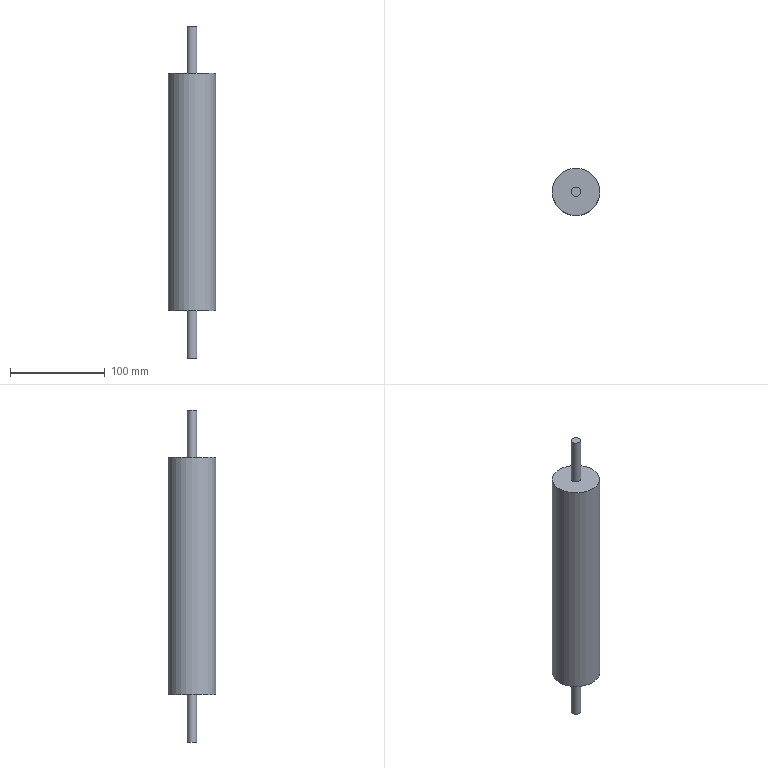Part | NX | 1 solid | 7 faces | box 50 x 50 x 350 mm | volume 498728 mm3 | plane 4 | cylinder 3 | commonest cylinder face diameters 10 x2 50 x1
STEP:
#1=CARTESIAN_POINT('',(-5.,0.,-175.));
#2=VERTEX_POINT('',#1);
#3=CARTESIAN_POINT('',(0.,0.,-175.));
#4=DIRECTION('',(0.,0.,1.));
#5=DIRECTION('',(-1.,0.,0.));
#6=AXIS2_PLACEMENT_3D('',#3,#4,#5);
#7=CIRCLE('',#6,5.);
#8=EDGE_CURVE('',#2,#2,#7,.T.);
#9=ORIENTED_EDGE('',*,*,#8,.F.);
#10=EDGE_LOOP('',(#9));
#11=FACE_OUTER_BOUND('',#10,.T.);
#12=CARTESIAN_POINT('',(0.,0.,-175.));
#13=DIRECTION('',(0.,0.,1.));
#14=DIRECTION('',(1.,0.,0.));
#15=AXIS2_PLACEMENT_3D('',#12,#13,#14);
#16=PLANE('',#15);
#17=ADVANCED_FACE('',(#11),#16,.F.);
#18=CARTESIAN_POINT('',(5.,0.,175.));
#19=VERTEX_POINT('',#18);
#20=CARTESIAN_POINT('',(0.,0.,175.));
#21=DIRECTION('',(0.,0.,1.));
#22=DIRECTION('',(-1.,0.,0.));
#23=AXIS2_PLACEMENT_3D('',#20,#21,#22);
#24=CIRCLE('',#23,5.);
#25=EDGE_CURVE('',#19,#19,#24,.T.);
#26=ORIENTED_EDGE('',*,*,#25,.T.);
#27=EDGE_LOOP('',(#26));
#28=FACE_OUTER_BOUND('',#27,.T.);
#29=CARTESIAN_POINT('',(0.,0.,175.));
#30=DIRECTION('',(0.,0.,1.));
#31=DIRECTION('',(1.,0.,0.));
#32=AXIS2_PLACEMENT_3D('',#29,#30,#31);
#33=PLANE('',#32);
#34=ADVANCED_FACE('',(#28),#33,.T.);
#35=CARTESIAN_POINT('',(25.,0.,-125.));
#36=VERTEX_POINT('',#35);
#37=CARTESIAN_POINT('',(0.,0.,-125.));
#38=DIRECTION('',(0.,0.,1.));
#39=DIRECTION('',(1.,0.,0.));
#40=AXIS2_PLACEMENT_3D('',#37,#38,#39);
#41=CIRCLE('',#40,25.);
#42=EDGE_CURVE('',#36,#36,#41,.T.);
#43=ORIENTED_EDGE('',*,*,#42,.T.);
#44=EDGE_LOOP('',(#43));
#45=FACE_BOUND('',#44,.T.);
#46=CARTESIAN_POINT('',(25.,0.,125.));
#47=VERTEX_POINT('',#46);
#48=CARTESIAN_POINT('',(0.,0.,125.));
#49=DIRECTION('',(0.,0.,1.));
#50=DIRECTION('',(1.,0.,0.));
#51=AXIS2_PLACEMENT_3D('',#48,#49,#50);
#52=CIRCLE('',#51,25.);
#53=EDGE_CURVE('',#47,#47,#52,.T.);
#54=ORIENTED_EDGE('',*,*,#53,.F.);
#55=EDGE_LOOP('',(#54));
#56=FACE_BOUND('',#55,.T.);
#57=CARTESIAN_POINT('',(0.,0.,-175.));
#58=DIRECTION('',(0.,0.,1.));
#59=DIRECTION('',(1.,0.,0.));
#60=AXIS2_PLACEMENT_3D('',#57,#58,#59);
#61=CYLINDRICAL_SURFACE('',#60,25.);
#62=ADVANCED_FACE('',(#45,#56),#61,.T.);
#63=ORIENTED_EDGE('',*,*,#53,.T.);
#64=EDGE_LOOP('',(#63));
#65=FACE_BOUND('',#64,.T.);
#66=CARTESIAN_POINT('',(5.,0.,125.));
#67=VERTEX_POINT('',#66);
#68=CARTESIAN_POINT('',(0.,0.,125.));
#69=DIRECTION('',(0.,0.,-1.));
#70=DIRECTION('',(1.,0.,0.));
#71=AXIS2_PLACEMENT_3D('',#68,#69,#70);
#72=CIRCLE('',#71,5.);
#73=EDGE_CURVE('',#67,#67,#72,.T.);
#74=ORIENTED_EDGE('',*,*,#73,.T.);
#75=EDGE_LOOP('',(#74));
#76=FACE_BOUND('',#75,.T.);
#77=CARTESIAN_POINT('',(0.,0.,125.));
#78=DIRECTION('',(0.,0.,1.));
#79=DIRECTION('',(1.,0.,0.));
#80=AXIS2_PLACEMENT_3D('',#77,#78,#79);
#81=PLANE('',#80);
#82=ADVANCED_FACE('',(#65,#76),#81,.T.);
#83=ORIENTED_EDGE('',*,*,#25,.F.);
#84=EDGE_LOOP('',(#83));
#85=FACE_BOUND('',#84,.T.);
#86=ORIENTED_EDGE('',*,*,#73,.F.);
#87=EDGE_LOOP('',(#86));
#88=FACE_BOUND('',#87,.T.);
#89=CARTESIAN_POINT('',(0.,0.,175.));
#90=DIRECTION('',(0.,0.,1.));
#91=DIRECTION('',(1.,0.,0.));
#92=AXIS2_PLACEMENT_3D('',#89,#90,#91);
#93=CYLINDRICAL_SURFACE('',#92,5.);
#94=ADVANCED_FACE('',(#85,#88),#93,.T.);
#95=ORIENTED_EDGE('',*,*,#42,.F.);
#96=EDGE_LOOP('',(#95));
#97=FACE_BOUND('',#96,.T.);
#98=CARTESIAN_POINT('',(-5.,0.,-125.));
#99=VERTEX_POINT('',#98);
#100=CARTESIAN_POINT('',(0.,0.,-125.));
#101=DIRECTION('',(0.,0.,-1.));
#102=DIRECTION('',(1.,0.,0.));
#103=AXIS2_PLACEMENT_3D('',#100,#101,#102);
#104=CIRCLE('',#103,5.);
#105=EDGE_CURVE('',#99,#99,#104,.T.);
#106=ORIENTED_EDGE('',*,*,#105,.F.);
#107=EDGE_LOOP('',(#106));
#108=FACE_BOUND('',#107,.T.);
#109=CARTESIAN_POINT('',(0.,0.,-125.));
#110=DIRECTION('',(0.,0.,1.));
#111=DIRECTION('',(1.,0.,0.));
#112=AXIS2_PLACEMENT_3D('',#109,#110,#111);
#113=PLANE('',#112);
#114=ADVANCED_FACE('',(#97,#108),#113,.F.);
#115=ORIENTED_EDGE('',*,*,#8,.T.);
#116=EDGE_LOOP('',(#115));
#117=FACE_BOUND('',#116,.T.);
#118=ORIENTED_EDGE('',*,*,#105,.T.);
#119=EDGE_LOOP('',(#118));
#120=FACE_BOUND('',#119,.T.);
#121=CARTESIAN_POINT('',(0.,0.,-175.));
#122=DIRECTION('',(0.,0.,1.));
#123=DIRECTION('',(1.,0.,0.));
#124=AXIS2_PLACEMENT_3D('',#121,#122,#123);
#125=CYLINDRICAL_SURFACE('',#124,5.);
#126=ADVANCED_FACE('',(#117,#120),#125,.T.);
#127=CLOSED_SHELL('',(#17,#34,#62,#82,#94,#114,#126));
#128=MANIFOLD_SOLID_BREP('',#127);
#129=(LENGTH_UNIT()NAMED_UNIT(*)SI_UNIT(.MILLI.,.METRE.));
#130=UNCERTAINTY_MEASURE_WITH_UNIT(LENGTH_MEASURE(0.00002),#129,'','');
#131=(NAMED_UNIT(*)PLANE_ANGLE_UNIT()SI_UNIT($,.RADIAN.));
#132=PLANE_ANGLE_MEASURE_WITH_UNIT(PLANE_ANGLE_MEASURE(0.01745),#131);
#133=DIMENSIONAL_EXPONENTS(0.,0.,0.,0.,0.,0.,0.);
#134=(CONVERSION_BASED_UNIT('DEGREE',#132)NAMED_UNIT(#133)PLANE_ANGLE_UNIT());
#135=(NAMED_UNIT(*)SI_UNIT($,.STERADIAN.)SOLID_ANGLE_UNIT());
#136=(GEOMETRIC_REPRESENTATION_CONTEXT(3)GLOBAL_UNCERTAINTY_ASSIGNED_CONTEXT((#130))GLOBAL_UNIT_ASSIGNED_CONTEXT((#129,#134,#135))REPRESENTATION_CONTEXT('',''));
#137=ADVANCED_BREP_SHAPE_REPRESENTATION('',(#128),#136);